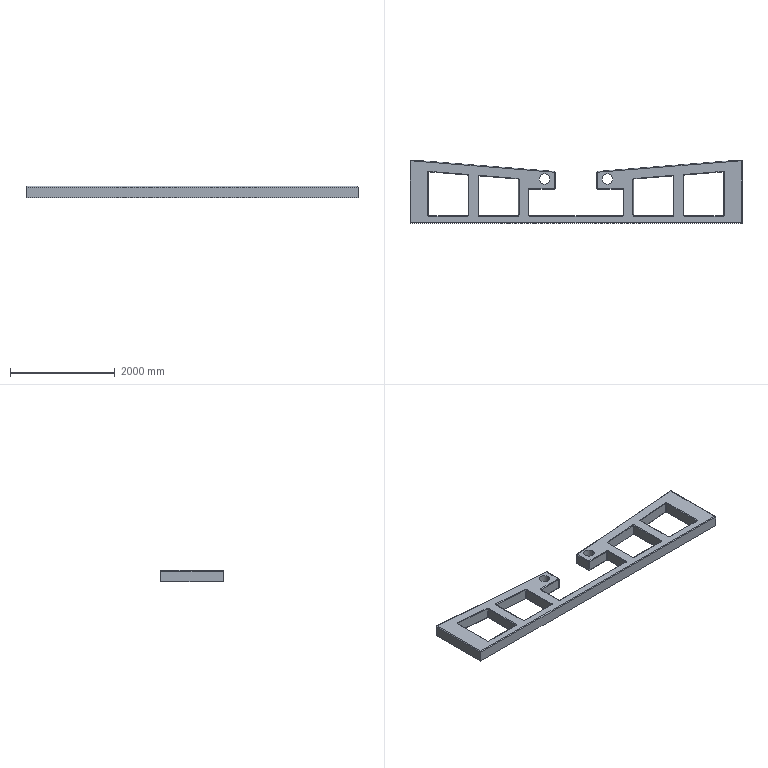Part | SolidWorks | features Fillet 8, ICE 3, Cut 2, Extrusion 1 | 1 solid | 161 faces | box 6350 x 1200 x 220 mm | volume 732765661 mm3 | cylinder 81 | torus 40 | plane 32 | sphere 8 | commonest cylinder face diameters 20 x48 30 x29 200 x4